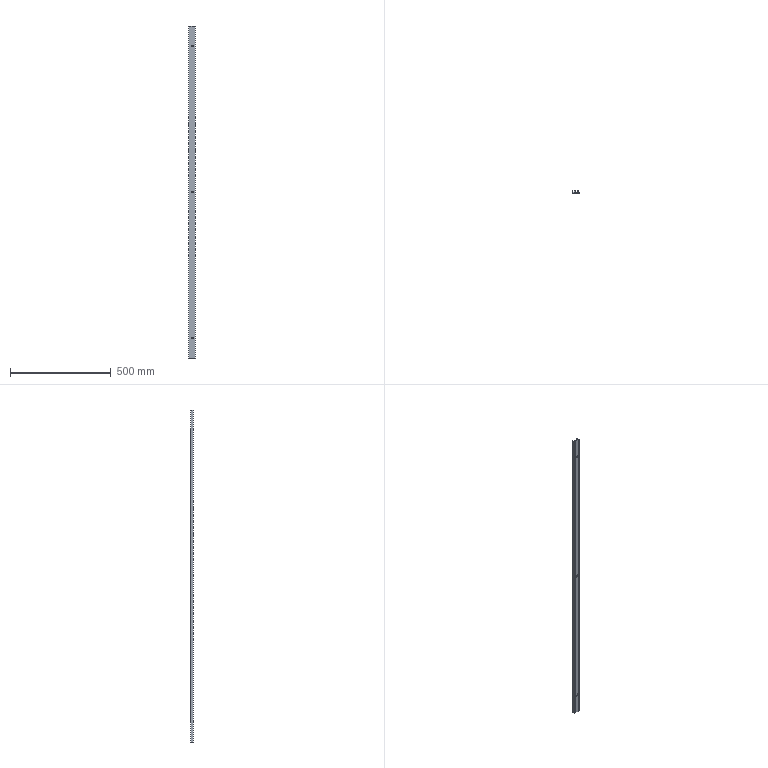Part | SolidWorks | features BaseBody 1, HoleWzd 1, ICE 1, MoveFace 1 | 1 solid | 31 faces | box 33.5 x 13.5 x 1650 mm | volume 308881 mm3 | plane 16 | cylinder 9 | cone 6 | commonest cylinder face diameters 2 x3 13.44 x3 4 x2 1.5 x1
STEP:
#1=CARTESIAN_POINT('',(20.,0.,1453.72));
#2=VERTEX_POINT('',#1);
#3=CARTESIAN_POINT('',(20.,0.,1446.28));
#4=VERTEX_POINT('',#3);
#5=CARTESIAN_POINT('',(20.,0.,1450.));
#6=DIRECTION('',(0.,-1.,0.));
#7=DIRECTION('',(0.,0.,-1.));
#8=AXIS2_PLACEMENT_3D('',#5,#6,#7);
#9=CIRCLE('',#8,3.72);
#10=EDGE_CURVE('',#2,#4,#9,.T.);
#11=ORIENTED_EDGE('',*,*,#10,.T.);
#12=CARTESIAN_POINT('',(20.,3.,1443.28));
#13=VERTEX_POINT('',#12);
#14=CARTESIAN_POINT('',(20.,3.,1443.28));
#15=DIRECTION('',(0.,0.7071,-0.7071));
#16=VECTOR('',#15,1000.);
#17=LINE('',#14,#16);
#18=EDGE_CURVE('',#4,#13,#17,.T.);
#19=ORIENTED_EDGE('',*,*,#18,.T.);
#20=CARTESIAN_POINT('',(20.,3.,1456.72));
#21=VERTEX_POINT('',#20);
#22=CARTESIAN_POINT('',(20.,3.,1450.));
#23=DIRECTION('',(0.,1.,0.));
#24=DIRECTION('',(0.,0.,1.));
#25=AXIS2_PLACEMENT_3D('',#22,#23,#24);
#26=CIRCLE('',#25,6.72);
#27=EDGE_CURVE('',#13,#21,#26,.T.);
#28=ORIENTED_EDGE('',*,*,#27,.T.);
#29=CARTESIAN_POINT('',(20.,3.,1456.72));
#30=DIRECTION('',(0.,0.7071,0.7071));
#31=VECTOR('',#30,1000.);
#32=LINE('',#29,#31);
#33=EDGE_CURVE('',#2,#21,#32,.T.);
#34=ORIENTED_EDGE('',*,*,#33,.F.);
#35=EDGE_LOOP('',(#11,#19,#28,#34));
#36=FACE_OUTER_BOUND('',#35,.T.);
#37=CARTESIAN_POINT('',(20.,3.,1450.));
#38=DIRECTION('',(0.,1.,0.));
#39=DIRECTION('',(0.,0.,1.));
#40=AXIS2_PLACEMENT_3D('',#37,#38,#39);
#41=CONICAL_SURFACE('',#40,6.72,0.7854);
#42=ADVANCED_FACE('',(#36),#41,.F.);
#43=CARTESIAN_POINT('',(20.,0.,3.72));
#44=VERTEX_POINT('',#43);
#45=CARTESIAN_POINT('',(20.,0.,-3.72));
#46=VERTEX_POINT('',#45);
#47=CARTESIAN_POINT('',(20.,0.,0.));
#48=DIRECTION('',(0.,-1.,0.));
#49=DIRECTION('',(0.,0.,-1.));
#50=AXIS2_PLACEMENT_3D('',#47,#48,#49);
#51=CIRCLE('',#50,3.72);
#52=EDGE_CURVE('',#44,#46,#51,.T.);
#53=ORIENTED_EDGE('',*,*,#52,.T.);
#54=CARTESIAN_POINT('',(20.,3.,-6.72));
#55=VERTEX_POINT('',#54);
#56=CARTESIAN_POINT('',(20.,3.,-6.72));
#57=DIRECTION('',(0.,0.7071,-0.7071));
#58=VECTOR('',#57,1000.);
#59=LINE('',#56,#58);
#60=EDGE_CURVE('',#46,#55,#59,.T.);
#61=ORIENTED_EDGE('',*,*,#60,.T.);
#62=CARTESIAN_POINT('',(20.,3.,6.72));
#63=VERTEX_POINT('',#62);
#64=CARTESIAN_POINT('',(20.,3.,0.));
#65=DIRECTION('',(0.,1.,0.));
#66=DIRECTION('',(0.,0.,1.));
#67=AXIS2_PLACEMENT_3D('',#64,#65,#66);
#68=CIRCLE('',#67,6.72);
#69=EDGE_CURVE('',#55,#63,#68,.T.);
#70=ORIENTED_EDGE('',*,*,#69,.T.);
#71=CARTESIAN_POINT('',(20.,3.,6.72));
#72=DIRECTION('',(0.,0.7071,0.7071));
#73=VECTOR('',#72,1000.);
#74=LINE('',#71,#73);
#75=EDGE_CURVE('',#44,#63,#74,.T.);
#76=ORIENTED_EDGE('',*,*,#75,.F.);
#77=EDGE_LOOP('',(#53,#61,#70,#76));
#78=FACE_OUTER_BOUND('',#77,.T.);
#79=CARTESIAN_POINT('',(20.,3.,0.));
#80=DIRECTION('',(0.,1.,0.));
#81=DIRECTION('',(0.,0.,1.));
#82=AXIS2_PLACEMENT_3D('',#79,#80,#81);
#83=CONICAL_SURFACE('',#82,6.72,0.7854);
#84=ADVANCED_FACE('',(#78),#83,.F.);
#85=CARTESIAN_POINT('',(20.,0.,728.72));
#86=VERTEX_POINT('',#85);
#87=CARTESIAN_POINT('',(20.,0.,721.28));
#88=VERTEX_POINT('',#87);
#89=CARTESIAN_POINT('',(20.,0.,725.));
#90=DIRECTION('',(0.,-1.,0.));
#91=DIRECTION('',(0.,0.,-1.));
#92=AXIS2_PLACEMENT_3D('',#89,#90,#91);
#93=CIRCLE('',#92,3.72);
#94=EDGE_CURVE('',#86,#88,#93,.T.);
#95=ORIENTED_EDGE('',*,*,#94,.T.);
#96=CARTESIAN_POINT('',(20.,3.,718.28));
#97=VERTEX_POINT('',#96);
#98=CARTESIAN_POINT('',(20.,3.,718.28));
#99=DIRECTION('',(0.,0.7071,-0.7071));
#100=VECTOR('',#99,1000.);
#101=LINE('',#98,#100);
#102=EDGE_CURVE('',#88,#97,#101,.T.);
#103=ORIENTED_EDGE('',*,*,#102,.T.);
#104=CARTESIAN_POINT('',(20.,3.,731.72));
#105=VERTEX_POINT('',#104);
#106=CARTESIAN_POINT('',(20.,3.,725.));
#107=DIRECTION('',(0.,1.,0.));
#108=DIRECTION('',(0.,0.,1.));
#109=AXIS2_PLACEMENT_3D('',#106,#107,#108);
#110=CIRCLE('',#109,6.72);
#111=EDGE_CURVE('',#97,#105,#110,.T.);
#112=ORIENTED_EDGE('',*,*,#111,.T.);
#113=CARTESIAN_POINT('',(20.,3.,731.72));
#114=DIRECTION('',(0.,0.7071,0.7071));
#115=VECTOR('',#114,1000.);
#116=LINE('',#113,#115);
#117=EDGE_CURVE('',#86,#105,#116,.T.);
#118=ORIENTED_EDGE('',*,*,#117,.F.);
#119=EDGE_LOOP('',(#95,#103,#112,#118));
#120=FACE_OUTER_BOUND('',#119,.T.);
#121=CARTESIAN_POINT('',(20.,3.,725.));
#122=DIRECTION('',(0.,1.,0.));
#123=DIRECTION('',(0.,0.,1.));
#124=AXIS2_PLACEMENT_3D('',#121,#122,#123);
#125=CONICAL_SURFACE('',#124,6.72,0.7854);
#126=ADVANCED_FACE('',(#120),#125,.F.);
#127=CARTESIAN_POINT('',(24.5,10.5,-4.991));
#128=VERTEX_POINT('',#127);
#129=CARTESIAN_POINT('',(24.5,10.5,-100.));
#130=VERTEX_POINT('',#129);
#131=CARTESIAN_POINT('',(24.5,10.5,-100.));
#132=DIRECTION('',(0.,0.,-1.));
#133=VECTOR('',#132,1000.);
#134=LINE('',#131,#133);
#135=EDGE_CURVE('',#128,#130,#134,.T.);
#136=ORIENTED_EDGE('',*,*,#135,.F.);
#137=CARTESIAN_POINT('',(24.5,10.5,4.991));
#138=VERTEX_POINT('',#137);
#139=CARTESIAN_POINT('',(24.5,10.5,-4.991));
#140=CARTESIAN_POINT('',(24.5,10.638,-4.991));
#141=CARTESIAN_POINT('',(24.515,10.777,-4.978));
#142=CARTESIAN_POINT('',(24.57,11.043,-4.927));
#143=CARTESIAN_POINT('',(24.611,11.171,-4.889));
#144=CARTESIAN_POINT('',(24.765,11.529,-4.74));
#145=CARTESIAN_POINT('',(24.907,11.728,-4.597));
#146=CARTESIAN_POINT('',(25.205,12.04,-4.256));
#147=CARTESIAN_POINT('',(25.365,12.156,-4.055));
#148=CARTESIAN_POINT('',(25.663,12.325,-3.627));
#149=CARTESIAN_POINT('',(25.806,12.38,-3.395));
#150=CARTESIAN_POINT('',(26.19,12.494,-2.672));
#151=CARTESIAN_POINT('',(26.387,12.501,-2.161));
#152=CARTESIAN_POINT('',(26.654,12.499,-1.091));
#153=CARTESIAN_POINT('',(26.72,12.488,-0.5481));
#154=CARTESIAN_POINT('',(26.72,12.488,0.2773));
#155=CARTESIAN_POINT('',(26.703,12.49,0.5529));
#156=CARTESIAN_POINT('',(26.636,12.496,1.095));
#157=CARTESIAN_POINT('',(26.586,12.499,1.362));
#158=CARTESIAN_POINT('',(26.388,12.501,2.155));
#159=CARTESIAN_POINT('',(26.188,12.493,2.677));
#160=CARTESIAN_POINT('',(25.805,12.38,3.396));
#161=CARTESIAN_POINT('',(25.662,12.324,3.629));
#162=CARTESIAN_POINT('',(25.438,12.197,3.95));
#163=CARTESIAN_POINT('',(25.362,12.147,4.053));
#164=CARTESIAN_POINT('',(25.208,12.03,4.249));
#165=CARTESIAN_POINT('',(25.13,11.961,4.342));
#166=CARTESIAN_POINT('',(24.98,11.805,4.513));
#167=CARTESIAN_POINT('',(24.908,11.717,4.591));
#168=CARTESIAN_POINT('',(24.774,11.518,4.73));
#169=CARTESIAN_POINT('',(24.714,11.408,4.79));
#170=CARTESIAN_POINT('',(24.612,11.172,4.888));
#171=CARTESIAN_POINT('',(24.57,11.043,4.927));
#172=CARTESIAN_POINT('',(24.515,10.778,4.978));
#173=CARTESIAN_POINT('',(24.5,10.64,4.991));
#174=CARTESIAN_POINT('',(24.5,10.5,4.991));
#175=B_SPLINE_CURVE_WITH_KNOTS('',3,(#139,#140,#141,#142,#143,#144,#145,#146,#147,#148,#149,#150,#151,#152,#153,#154,#155,#156,#157,#158,#159,#160,#161,#162,#163,#164,#165,#166,#167,#168,#169,#170,#171,#172,#173,#174),.UNSPECIFIED.,.F.,.F.,(4,2,2,2,2,2,2,2,2,2,2,2,2,2,2,2,2,4),(0.01321,0.01362,0.01403,0.01486,0.01569,0.01651,0.01816,0.01981,0.02064,0.02146,0.02311,0.02394,0.02435,0.02477,0.02518,0.02559,0.026,0.02642),.UNSPECIFIED.);
#176=EDGE_CURVE('',#128,#138,#175,.T.);
#177=ORIENTED_EDGE('',*,*,#176,.T.);
#178=CARTESIAN_POINT('',(24.5,10.5,720.009));
#179=VERTEX_POINT('',#178);
#180=CARTESIAN_POINT('',(24.5,10.5,-100.));
#181=DIRECTION('',(0.,0.,-1.));
#182=VECTOR('',#181,1000.);
#183=LINE('',#180,#182);
#184=EDGE_CURVE('',#179,#138,#183,.T.);
#185=ORIENTED_EDGE('',*,*,#184,.F.);
#186=CARTESIAN_POINT('',(24.5,10.5,729.991));
#187=VERTEX_POINT('',#186);
#188=CARTESIAN_POINT('',(24.5,10.5,720.009));
#189=CARTESIAN_POINT('',(24.5,10.638,720.009));
#190=CARTESIAN_POINT('',(24.515,10.777,720.022));
#191=CARTESIAN_POINT('',(24.57,11.043,720.073));
#192=CARTESIAN_POINT('',(24.611,11.171,720.111));
#193=CARTESIAN_POINT('',(24.765,11.529,720.26));
#194=CARTESIAN_POINT('',(24.907,11.728,720.403));
#195=CARTESIAN_POINT('',(25.205,12.04,720.744));
#196=CARTESIAN_POINT('',(25.365,12.156,720.945));
#197=CARTESIAN_POINT('',(25.663,12.325,721.373));
#198=CARTESIAN_POINT('',(25.806,12.38,721.605));
#199=CARTESIAN_POINT('',(26.19,12.494,722.328));
#200=CARTESIAN_POINT('',(26.387,12.501,722.839));
#201=CARTESIAN_POINT('',(26.654,12.499,723.909));
#202=CARTESIAN_POINT('',(26.72,12.488,724.452));
#203=CARTESIAN_POINT('',(26.72,12.488,725.277));
#204=CARTESIAN_POINT('',(26.703,12.49,725.553));
#205=CARTESIAN_POINT('',(26.636,12.496,726.095));
#206=CARTESIAN_POINT('',(26.586,12.499,726.362));
#207=CARTESIAN_POINT('',(26.388,12.501,727.155));
#208=CARTESIAN_POINT('',(26.188,12.493,727.677));
#209=CARTESIAN_POINT('',(25.805,12.38,728.396));
#210=CARTESIAN_POINT('',(25.662,12.324,728.629));
#211=CARTESIAN_POINT('',(25.438,12.197,728.95));
#212=CARTESIAN_POINT('',(25.362,12.147,729.053));
#213=CARTESIAN_POINT('',(25.208,12.03,729.249));
#214=CARTESIAN_POINT('',(25.13,11.961,729.342));
#215=CARTESIAN_POINT('',(24.98,11.805,729.513));
#216=CARTESIAN_POINT('',(24.908,11.717,729.591));
#217=CARTESIAN_POINT('',(24.774,11.518,729.73));
#218=CARTESIAN_POINT('',(24.714,11.408,729.79));
#219=CARTESIAN_POINT('',(24.612,11.172,729.888));
#220=CARTESIAN_POINT('',(24.57,11.043,729.927));
#221=CARTESIAN_POINT('',(24.515,10.778,729.978));
#222=CARTESIAN_POINT('',(24.5,10.64,729.991));
#223=CARTESIAN_POINT('',(24.5,10.5,729.991));
#224=B_SPLINE_CURVE_WITH_KNOTS('',3,(#188,#189,#190,#191,#192,#193,#194,#195,#196,#197,#198,#199,#200,#201,#202,#203,#204,#205,#206,#207,#208,#209,#210,#211,#212,#213,#214,#215,#216,#217,#218,#219,#220,#221,#222,#223),.UNSPECIFIED.,.F.,.F.,(4,2,2,2,2,2,2,2,2,2,2,2,2,2,2,2,2,4),(0.01321,0.01362,0.01403,0.01486,0.01569,0.01651,0.01816,0.01981,0.02064,0.02146,0.02311,0.02394,0.02435,0.02477,0.02518,0.02559,0.026,0.02642),.UNSPECIFIED.);
#225=EDGE_CURVE('',#179,#187,#224,.T.);
#226=ORIENTED_EDGE('',*,*,#225,.T.);
#227=CARTESIAN_POINT('',(24.5,10.5,1445.009));
#228=VERTEX_POINT('',#227);
#229=CARTESIAN_POINT('',(24.5,10.5,-100.));
#230=DIRECTION('',(0.,0.,-1.));
#231=VECTOR('',#230,1000.);
#232=LINE('',#229,#231);
#233=EDGE_CURVE('',#228,#187,#232,.T.);
#234=ORIENTED_EDGE('',*,*,#233,.F.);
#235=CARTESIAN_POINT('',(24.5,10.5,1454.991));
#236=VERTEX_POINT('',#235);
#237=CARTESIAN_POINT('',(24.5,10.5,1445.009));
#238=CARTESIAN_POINT('',(24.5,10.64,1445.009));
#239=CARTESIAN_POINT('',(24.514,10.776,1445.022));
#240=CARTESIAN_POINT('',(24.57,11.042,1445.073));
#241=CARTESIAN_POINT('',(24.611,11.171,1445.111));
#242=CARTESIAN_POINT('',(24.713,11.408,1445.209));
#243=CARTESIAN_POINT('',(24.775,11.519,1445.27));
#244=CARTESIAN_POINT('',(24.908,11.717,1445.409));
#245=CARTESIAN_POINT('',(24.981,11.806,1445.488));
#246=CARTESIAN_POINT('',(25.207,12.042,1445.746));
#247=CARTESIAN_POINT('',(25.363,12.155,1445.942));
#248=CARTESIAN_POINT('',(25.665,12.326,1446.376));
#249=CARTESIAN_POINT('',(25.806,12.38,1446.605));
#250=CARTESIAN_POINT('',(26.061,12.456,1447.084));
#251=CARTESIAN_POINT('',(26.176,12.476,1447.337));
#252=CARTESIAN_POINT('',(26.372,12.498,1447.849));
#253=CARTESIAN_POINT('',(26.454,12.501,1448.109));
#254=CARTESIAN_POINT('',(26.586,12.499,1448.638));
#255=CARTESIAN_POINT('',(26.636,12.496,1448.907));
#256=CARTESIAN_POINT('',(26.703,12.49,1449.453));
#257=CARTESIAN_POINT('',(26.72,12.488,1449.729));
#258=CARTESIAN_POINT('',(26.72,12.488,1450.275));
#259=CARTESIAN_POINT('',(26.703,12.49,1450.547));
#260=CARTESIAN_POINT('',(26.637,12.496,1451.089));
#261=CARTESIAN_POINT('',(26.587,12.499,1451.36));
#262=CARTESIAN_POINT('',(26.387,12.501,1452.161));
#263=CARTESIAN_POINT('',(26.191,12.494,1452.671));
#264=CARTESIAN_POINT('',(25.805,12.38,1453.396));
#265=CARTESIAN_POINT('',(25.663,12.325,1453.627));
#266=CARTESIAN_POINT('',(25.364,12.155,1454.057));
#267=CARTESIAN_POINT('',(25.205,12.039,1454.256));
#268=CARTESIAN_POINT('',(24.981,11.805,1454.512));
#269=CARTESIAN_POINT('',(24.907,11.716,1454.592));
#270=CARTESIAN_POINT('',(24.774,11.518,1454.73));
#271=CARTESIAN_POINT('',(24.714,11.409,1454.79));
#272=CARTESIAN_POINT('',(24.611,11.17,1454.889));
#273=CARTESIAN_POINT('',(24.571,11.044,1454.926));
#274=CARTESIAN_POINT('',(24.515,10.78,1454.977));
#275=CARTESIAN_POINT('',(24.5,10.64,1454.991));
#276=CARTESIAN_POINT('',(24.5,10.5,1454.991));
#277=B_SPLINE_CURVE_WITH_KNOTS('',3,(#237,#238,#239,#240,#241,#242,#243,#244,#245,#246,#247,#248,#249,#250,#251,#252,#253,#254,#255,#256,#257,#258,#259,#260,#261,#262,#263,#264,#265,#266,#267,#268,#269,#270,#271,#272,#273,#274,#275,#276),.UNSPECIFIED.,.F.,.F.,(4,2,2,2,2,2,2,2,2,2,2,2,2,2,2,2,2,2,2,4),(0.,0.0004127,0.0008255,0.001238,0.001651,0.002476,0.003302,0.004127,0.004953,0.005778,0.006604,0.007429,0.008255,0.009906,0.01073,0.01156,0.01197,0.01238,0.01279,0.01321),.UNSPECIFIED.);
#278=EDGE_CURVE('',#228,#236,#277,.T.);
#279=ORIENTED_EDGE('',*,*,#278,.T.);
#280=CARTESIAN_POINT('',(24.5,10.5,1550.));
#281=VERTEX_POINT('',#280);
#282=CARTESIAN_POINT('',(24.5,10.5,-100.));
#283=DIRECTION('',(0.,0.,-1.));
#284=VECTOR('',#283,1000.);
#285=LINE('',#282,#284);
#286=EDGE_CURVE('',#281,#236,#285,.T.);
#287=ORIENTED_EDGE('',*,*,#286,.F.);
#288=CARTESIAN_POINT('',(28.5,10.5,1550.));
#289=VERTEX_POINT('',#288);
#290=CARTESIAN_POINT('',(26.5,10.5,1550.));
#291=DIRECTION('',(0.,0.,1.));
#292=DIRECTION('',(1.,0.,0.));
#293=AXIS2_PLACEMENT_3D('',#290,#291,#292);
#294=CIRCLE('',#293,2.);
#295=EDGE_CURVE('',#289,#281,#294,.T.);
#296=ORIENTED_EDGE('',*,*,#295,.F.);
#297=CARTESIAN_POINT('',(28.5,10.5,-100.));
#298=VERTEX_POINT('',#297);
#299=CARTESIAN_POINT('',(28.5,10.5,-100.));
#300=DIRECTION('',(0.,0.,-1.));
#301=VECTOR('',#300,1000.);
#302=LINE('',#299,#301);
#303=EDGE_CURVE('',#289,#298,#302,.T.);
#304=ORIENTED_EDGE('',*,*,#303,.T.);
#305=CARTESIAN_POINT('',(26.5,10.5,-100.));
#306=DIRECTION('',(0.,0.,1.));
#307=DIRECTION('',(-1.,0.,0.));
#308=AXIS2_PLACEMENT_3D('',#305,#306,#307);
#309=CIRCLE('',#308,2.);
#310=EDGE_CURVE('',#298,#130,#309,.T.);
#311=ORIENTED_EDGE('',*,*,#310,.T.);
#312=EDGE_LOOP('',(#136,#177,#185,#226,#234,#279,#287,#296,#304,#311));
#313=FACE_OUTER_BOUND('',#312,.T.);
#314=CARTESIAN_POINT('',(26.5,10.5,-100.));
#315=DIRECTION('',(0.,0.,-1.));
#316=DIRECTION('',(-1.,0.,0.));
#317=AXIS2_PLACEMENT_3D('',#314,#315,#316);
#318=CYLINDRICAL_SURFACE('',#317,2.);
#319=ADVANCED_FACE('',(#313),#318,.T.);
#320=CARTESIAN_POINT('',(24.5,3.,-4.991));
#321=VERTEX_POINT('',#320);
#322=CARTESIAN_POINT('',(24.5,3.,-100.));
#323=VERTEX_POINT('',#322);
#324=CARTESIAN_POINT('',(24.5,3.,-100.));
#325=DIRECTION('',(0.,0.,-1.));
#326=VECTOR('',#325,1000.);
#327=LINE('',#324,#326);
#328=EDGE_CURVE('',#321,#323,#327,.T.);
#329=ORIENTED_EDGE('',*,*,#328,.F.);
#330=CARTESIAN_POINT('',(24.5,13.5,-4.991));
#331=DIRECTION('',(0.,1.,0.));
#332=VECTOR('',#331,1000.);
#333=LINE('',#330,#332);
#334=EDGE_CURVE('',#321,#128,#333,.T.);
#335=ORIENTED_EDGE('',*,*,#334,.T.);
#336=ORIENTED_EDGE('',*,*,#135,.T.);
#337=CARTESIAN_POINT('',(24.5,1.,-100.));
#338=DIRECTION('',(0.,-1.,0.));
#339=VECTOR('',#338,1000.);
#340=LINE('',#337,#339);
#341=EDGE_CURVE('',#130,#323,#340,.T.);
#342=ORIENTED_EDGE('',*,*,#341,.T.);
#343=EDGE_LOOP('',(#329,#335,#336,#342));
#344=FACE_OUTER_BOUND('',#343,.T.);
#345=CARTESIAN_POINT('',(24.5,10.5,-100.));
#346=DIRECTION('',(-1.,0.,0.));
#347=DIRECTION('',(0.,0.,1.));
#348=AXIS2_PLACEMENT_3D('',#345,#346,#347);
#349=PLANE('',#348);
#350=ADVANCED_FACE('',(#344),#349,.T.);
#351=ORIENTED_EDGE('',*,*,#184,.T.);
#352=CARTESIAN_POINT('',(24.5,3.,4.991));
#353=VERTEX_POINT('',#352);
#354=CARTESIAN_POINT('',(24.5,13.5,4.991));
#355=DIRECTION('',(0.,-1.,0.));
#356=VECTOR('',#355,1000.);
#357=LINE('',#354,#356);
#358=EDGE_CURVE('',#138,#353,#357,.T.);
#359=ORIENTED_EDGE('',*,*,#358,.T.);
#360=CARTESIAN_POINT('',(24.5,3.,720.009));
#361=VERTEX_POINT('',#360);
#362=CARTESIAN_POINT('',(24.5,3.,-100.));
#363=DIRECTION('',(0.,0.,-1.));
#364=VECTOR('',#363,1000.);
#365=LINE('',#362,#364);
#366=EDGE_CURVE('',#361,#353,#365,.T.);
#367=ORIENTED_EDGE('',*,*,#366,.F.);
#368=CARTESIAN_POINT('',(24.5,13.5,720.009));
#369=DIRECTION('',(0.,1.,0.));
#370=VECTOR('',#369,1000.);
#371=LINE('',#368,#370);
#372=EDGE_CURVE('',#361,#179,#371,.T.);
#373=ORIENTED_EDGE('',*,*,#372,.T.);
#374=EDGE_LOOP('',(#351,#359,#367,#373));
#375=FACE_OUTER_BOUND('',#374,.T.);
#376=CARTESIAN_POINT('',(24.5,10.5,-100.));
#377=DIRECTION('',(-1.,0.,0.));
#378=DIRECTION('',(0.,0.,1.));
#379=AXIS2_PLACEMENT_3D('',#376,#377,#378);
#380=PLANE('',#379);
#381=ADVANCED_FACE('',(#375),#380,.T.);
#382=ORIENTED_EDGE('',*,*,#233,.T.);
#383=CARTESIAN_POINT('',(24.5,3.,729.991));
#384=VERTEX_POINT('',#383);
#385=CARTESIAN_POINT('',(24.5,13.5,729.991));
#386=DIRECTION('',(0.,-1.,0.));
#387=VECTOR('',#386,1000.);
#388=LINE('',#385,#387);
#389=EDGE_CURVE('',#187,#384,#388,.T.);
#390=ORIENTED_EDGE('',*,*,#389,.T.);
#391=CARTESIAN_POINT('',(24.5,3.,1445.009));
#392=VERTEX_POINT('',#391);
#393=CARTESIAN_POINT('',(24.5,3.,-100.));
#394=DIRECTION('',(0.,0.,-1.));
#395=VECTOR('',#394,1000.);
#396=LINE('',#393,#395);
#397=EDGE_CURVE('',#392,#384,#396,.T.);
#398=ORIENTED_EDGE('',*,*,#397,.F.);
#399=CARTESIAN_POINT('',(24.5,13.5,1445.009));
#400=DIRECTION('',(0.,1.,0.));
#401=VECTOR('',#400,1000.);
#402=LINE('',#399,#401);
#403=EDGE_CURVE('',#392,#228,#402,.T.);
#404=ORIENTED_EDGE('',*,*,#403,.T.);
#405=EDGE_LOOP('',(#382,#390,#398,#404));
#406=FACE_OUTER_BOUND('',#405,.T.);
#407=CARTESIAN_POINT('',(24.5,10.5,-100.));
#408=DIRECTION('',(-1.,0.,0.));
#409=DIRECTION('',(0.,0.,1.));
#410=AXIS2_PLACEMENT_3D('',#407,#408,#409);
#411=PLANE('',#410);
#412=ADVANCED_FACE('',(#406),#411,.T.);
#413=ORIENTED_EDGE('',*,*,#286,.T.);
#414=CARTESIAN_POINT('',(24.5,3.,1454.991));
#415=VERTEX_POINT('',#414);
#416=CARTESIAN_POINT('',(24.5,13.5,1454.991));
#417=DIRECTION('',(0.,-1.,0.));
#418=VECTOR('',#417,1000.);
#419=LINE('',#416,#418);
#420=EDGE_CURVE('',#236,#415,#419,.T.);
#421=ORIENTED_EDGE('',*,*,#420,.T.);
#422=CARTESIAN_POINT('',(24.5,3.,1550.));
#423=VERTEX_POINT('',#422);
#424=CARTESIAN_POINT('',(24.5,3.,-100.));
#425=DIRECTION('',(0.,0.,-1.));
#426=VECTOR('',#425,1000.);
#427=LINE('',#424,#426);
#428=EDGE_CURVE('',#423,#415,#427,.T.);
#429=ORIENTED_EDGE('',*,*,#428,.F.);
#430=CARTESIAN_POINT('',(24.5,1.,1550.));
#431=DIRECTION('',(0.,-1.,0.));
#432=VECTOR('',#431,1000.);
#433=LINE('',#430,#432);
#434=EDGE_CURVE('',#281,#423,#433,.T.);
#435=ORIENTED_EDGE('',*,*,#434,.F.);
#436=EDGE_LOOP('',(#413,#421,#429,#435));
#437=FACE_OUTER_BOUND('',#436,.T.);
#438=CARTESIAN_POINT('',(24.5,10.5,-100.));
#439=DIRECTION('',(-1.,0.,0.));
#440=DIRECTION('',(0.,0.,1.));
#441=AXIS2_PLACEMENT_3D('',#438,#439,#440);
#442=PLANE('',#441);
#443=ADVANCED_FACE('',(#437),#442,.T.);
#444=ORIENTED_EDGE('',*,*,#10,.F.);
#445=CARTESIAN_POINT('',(20.,0.,1450.));
#446=DIRECTION('',(0.,-1.,0.));
#447=DIRECTION('',(0.,0.,-1.));
#448=AXIS2_PLACEMENT_3D('',#445,#446,#447);
#449=CIRCLE('',#448,3.72);
#450=EDGE_CURVE('',#4,#2,#449,.T.);
#451=ORIENTED_EDGE('',*,*,#450,.F.);
#452=EDGE_LOOP('',(#444,#451));
#453=FACE_BOUND('',#452,.T.);
#454=ORIENTED_EDGE('',*,*,#52,.F.);
#455=CARTESIAN_POINT('',(20.,0.,0.));
#456=DIRECTION('',(0.,-1.,0.));
#457=DIRECTION('',(0.,0.,-1.));
#458=AXIS2_PLACEMENT_3D('',#455,#456,#457);
#459=CIRCLE('',#458,3.72);
#460=EDGE_CURVE('',#46,#44,#459,.T.);
#461=ORIENTED_EDGE('',*,*,#460,.F.);
#462=EDGE_LOOP('',(#454,#461));
#463=FACE_BOUND('',#462,.T.);
#464=CARTESIAN_POINT('',(1.,0.,-100.));
#465=VERTEX_POINT('',#464);
#466=CARTESIAN_POINT('',(32.5,0.,-100.));
#467=VERTEX_POINT('',#466);
#468=CARTESIAN_POINT('',(1.,0.,-100.));
#469=DIRECTION('',(1.,0.,0.));
#470=VECTOR('',#469,1000.);
#471=LINE('',#468,#470);
#472=EDGE_CURVE('',#465,#467,#471,.T.);
#473=ORIENTED_EDGE('',*,*,#472,.T.);
#474=CARTESIAN_POINT('',(32.5,0.,1550.));
#475=VERTEX_POINT('',#474);
#476=CARTESIAN_POINT('',(32.5,0.,-100.));
#477=DIRECTION('',(0.,0.,1.));
#478=VECTOR('',#477,1000.);
#479=LINE('',#476,#478);
#480=EDGE_CURVE('',#467,#475,#479,.T.);
#481=ORIENTED_EDGE('',*,*,#480,.T.);
#482=CARTESIAN_POINT('',(1.,0.,1550.));
#483=VERTEX_POINT('',#482);
#484=CARTESIAN_POINT('',(1.,0.,1550.));
#485=DIRECTION('',(-1.,0.,0.));
#486=VECTOR('',#485,1000.);
#487=LINE('',#484,#486);
#488=EDGE_CURVE('',#475,#483,#487,.T.);
#489=ORIENTED_EDGE('',*,*,#488,.T.);
#490=CARTESIAN_POINT('',(1.,0.,-100.));
#491=DIRECTION('',(0.,0.,-1.));
#492=VECTOR('',#491,1000.);
#493=LINE('',#490,#492);
#494=EDGE_CURVE('',#483,#465,#493,.T.);
#495=ORIENTED_EDGE('',*,*,#494,.T.);
#496=EDGE_LOOP('',(#473,#481,#489,#495));
#497=FACE_OUTER_BOUND('',#496,.T.);
#498=ORIENTED_EDGE('',*,*,#94,.F.);
#499=CARTESIAN_POINT('',(20.,0.,725.));
#500=DIRECTION('',(0.,-1.,0.));
#501=DIRECTION('',(0.,0.,-1.));
#502=AXIS2_PLACEMENT_3D('',#499,#500,#501);
#503=CIRCLE('',#502,3.72);
#504=EDGE_CURVE('',#88,#86,#503,.T.);
#505=ORIENTED_EDGE('',*,*,#504,.F.);
#506=EDGE_LOOP('',(#498,#505));
#507=FACE_BOUND('',#506,.T.);
#508=CARTESIAN_POINT('',(1.,0.,-100.));
#509=DIRECTION('',(0.,-1.,0.));
#510=DIRECTION('',(0.,0.,-1.));
#511=AXIS2_PLACEMENT_3D('',#508,#509,#510);
#512=PLANE('',#511);
#513=ADVANCED_FACE('',(#453,#463,#497,#507),#512,.T.);
#514=CARTESIAN_POINT('',(33.5,1.,-100.));
#515=VERTEX_POINT('',#514);
#516=CARTESIAN_POINT('',(32.5,1.,-100.));
#517=DIRECTION('',(0.,0.,1.));
#518=DIRECTION('',(-1.,0.,0.));
#519=AXIS2_PLACEMENT_3D('',#516,#517,#518);
#520=CIRCLE('',#519,1.);
#521=EDGE_CURVE('',#467,#515,#520,.T.);
#522=ORIENTED_EDGE('',*,*,#521,.T.);
#523=CARTESIAN_POINT('',(33.5,1.,1550.));
#524=VERTEX_POINT('',#523);
#525=CARTESIAN_POINT('',(33.5,1.,-100.));
#526=DIRECTION('',(0.,0.,1.));
#527=VECTOR('',#526,1000.);
#528=LINE('',#525,#527);
#529=EDGE_CURVE('',#515,#524,#528,.T.);
#530=ORIENTED_EDGE('',*,*,#529,.T.);
#531=CARTESIAN_POINT('',(32.5,1.,1550.));
#532=DIRECTION('',(0.,0.,-1.));
#533=DIRECTION('',(1.,0.,0.));
#534=AXIS2_PLACEMENT_3D('',#531,#532,#533);
#535=CIRCLE('',#534,1.);
#536=EDGE_CURVE('',#524,#475,#535,.T.);
#537=ORIENTED_EDGE('',*,*,#536,.T.);
#538=ORIENTED_EDGE('',*,*,#480,.F.);
#539=EDGE_LOOP('',(#522,#530,#537,#538));
#540=FACE_OUTER_BOUND('',#539,.T.);
#541=CARTESIAN_POINT('',(32.5,1.,-100.));
#542=DIRECTION('',(0.,0.,-1.));
#543=DIRECTION('',(-1.,0.,0.));
#544=AXIS2_PLACEMENT_3D('',#541,#542,#543);
#545=CYLINDRICAL_SURFACE('',#544,1.);
#546=ADVANCED_FACE('',(#540),#545,.T.);
#547=CARTESIAN_POINT('',(1.5,12.75,-100.));
#548=VERTEX_POINT('',#547);
#549=CARTESIAN_POINT('',(0.,12.75,-100.));
#550=VERTEX_POINT('',#549);
#551=CARTESIAN_POINT('',(0.75,12.75,-100.));
#552=DIRECTION('',(0.,0.,1.));
#553=DIRECTION('',(-1.,0.,0.));
#554=AXIS2_PLACEMENT_3D('',#551,#552,#553);
#555=CIRCLE('',#554,0.75);
#556=EDGE_CURVE('',#548,#550,#555,.T.);
#557=ORIENTED_EDGE('',*,*,#556,.F.);
#558=CARTESIAN_POINT('',(1.5,3.,-100.));
#559=VERTEX_POINT('',#558);
#560=CARTESIAN_POINT('',(1.5,1.,-100.));
#561=DIRECTION('',(0.,1.,0.));
#562=VECTOR('',#561,1000.);
#563=LINE('',#560,#562);
#564=EDGE_CURVE('',#559,#548,#563,.T.);
#565=ORIENTED_EDGE('',*,*,#564,.F.);
#566=CARTESIAN_POINT('',(8.5,3.,-100.));
#567=VERTEX_POINT('',#566);
#568=CARTESIAN_POINT('',(1.,3.,-100.));
#569=DIRECTION('',(-1.,0.,0.));
#570=VECTOR('',#569,1000.);
#571=LINE('',#568,#570);
#572=EDGE_CURVE('',#567,#559,#571,.T.);
#573=ORIENTED_EDGE('',*,*,#572,.F.);
#574=CARTESIAN_POINT('',(8.5,10.5,-100.));
#575=VERTEX_POINT('',#574);
#576=CARTESIAN_POINT('',(8.5,1.,-100.));
#577=DIRECTION('',(0.,-1.,0.));
#578=VECTOR('',#577,1000.);
#579=LINE('',#576,#578);
#580=EDGE_CURVE('',#575,#567,#579,.T.);
#581=ORIENTED_EDGE('',*,*,#580,.F.);
#582=CARTESIAN_POINT('',(12.5,10.5,-100.));
#583=VERTEX_POINT('',#582);
#584=CARTESIAN_POINT('',(10.5,10.5,-100.));
#585=DIRECTION('',(0.,0.,1.));
#586=DIRECTION('',(-1.,0.,0.));
#587=AXIS2_PLACEMENT_3D('',#584,#585,#586);
#588=CIRCLE('',#587,2.);
#589=EDGE_CURVE('',#583,#575,#588,.T.);
#590=ORIENTED_EDGE('',*,*,#589,.F.);
#591=CARTESIAN_POINT('',(12.5,3.,-100.));
#592=VERTEX_POINT('',#591);
#593=CARTESIAN_POINT('',(12.5,1.,-100.));
#594=DIRECTION('',(0.,1.,0.));
#595=VECTOR('',#594,1000.);
#596=LINE('',#593,#595);
#597=EDGE_CURVE('',#592,#583,#596,.T.);
#598=ORIENTED_EDGE('',*,*,#597,.F.);
#599=CARTESIAN_POINT('',(1.,3.,-100.));
#600=DIRECTION('',(-1.,0.,0.));
#601=VECTOR('',#600,1000.);
#602=LINE('',#599,#601);
#603=EDGE_CURVE('',#323,#592,#602,.T.);
#604=ORIENTED_EDGE('',*,*,#603,.F.);
#605=ORIENTED_EDGE('',*,*,#341,.F.);
#606=ORIENTED_EDGE('',*,*,#310,.F.);
#607=CARTESIAN_POINT('',(28.5,3.,-100.));
#608=VERTEX_POINT('',#607);
#609=CARTESIAN_POINT('',(28.5,1.,-100.));
#610=DIRECTION('',(0.,1.,0.));
#611=VECTOR('',#610,1000.);
#612=LINE('',#609,#611);
#613=EDGE_CURVE('',#608,#298,#612,.T.);
#614=ORIENTED_EDGE('',*,*,#613,.F.);
#615=CARTESIAN_POINT('',(32.5,3.,-100.));
#616=VERTEX_POINT('',#615);
#617=CARTESIAN_POINT('',(1.,3.,-100.));
#618=DIRECTION('',(-1.,0.,0.));
#619=VECTOR('',#618,1000.);
#620=LINE('',#617,#619);
#621=EDGE_CURVE('',#616,#608,#620,.T.);
#622=ORIENTED_EDGE('',*,*,#621,.F.);
#623=CARTESIAN_POINT('',(33.5,2.,-100.));
#624=VERTEX_POINT('',#623);
#625=CARTESIAN_POINT('',(32.5,2.,-100.));
#626=DIRECTION('',(0.,0.,1.));
#627=DIRECTION('',(-1.,0.,0.));
#628=AXIS2_PLACEMENT_3D('',#625,#626,#627);
#629=CIRCLE('',#628,1.);
#630=EDGE_CURVE('',#624,#616,#629,.T.);
#631=ORIENTED_EDGE('',*,*,#630,.F.);
#632=CARTESIAN_POINT('',(33.5,1.,-100.));
#633=DIRECTION('',(0.,1.,0.));
#634=VECTOR('',#633,1000.);
#635=LINE('',#632,#634);
#636=EDGE_CURVE('',#515,#624,#635,.T.);
#637=ORIENTED_EDGE('',*,*,#636,.F.);
#638=ORIENTED_EDGE('',*,*,#521,.F.);
#639=ORIENTED_EDGE('',*,*,#472,.F.);
#640=CARTESIAN_POINT('',(0.,1.,-100.));
#641=VERTEX_POINT('',#640);
#642=CARTESIAN_POINT('',(1.,1.,-100.));
#643=DIRECTION('',(0.,0.,1.));
#644=DIRECTION('',(-1.,0.,0.));
#645=AXIS2_PLACEMENT_3D('',#642,#643,#644);
#646=CIRCLE('',#645,1.);
#647=EDGE_CURVE('',#641,#465,#646,.T.);
#648=ORIENTED_EDGE('',*,*,#647,.F.);
#649=CARTESIAN_POINT('',(0.,1.,-100.));
#650=DIRECTION('',(0.,-1.,0.));
#651=VECTOR('',#650,1000.);
#652=LINE('',#649,#651);
#653=EDGE_CURVE('',#550,#641,#652,.T.);
#654=ORIENTED_EDGE('',*,*,#653,.F.);
#655=EDGE_LOOP('',(#557,#565,#573,#581,#590,#598,#604,#605,#606,#614,#622,#631,#637,#638,#639,#648,#654));
#656=FACE_OUTER_BOUND('',#655,.T.);
#657=CARTESIAN_POINT('',(1.,1.,-100.));
#658=DIRECTION('',(0.,0.,1.));
#659=DIRECTION('',(1.,0.,0.));
#660=AXIS2_PLACEMENT_3D('',#657,#658,#659);
#661=PLANE('',#660);
#662=ADVANCED_FACE('',(#656),#661,.F.);
#663=ORIENTED_EDGE('',*,*,#647,.T.);
#664=ORIENTED_EDGE('',*,*,#494,.F.);
#665=CARTESIAN_POINT('',(0.,1.,1550.));
#666=VERTEX_POINT('',#665);
#667=CARTESIAN_POINT('',(1.,1.,1550.));
#668=DIRECTION('',(0.,0.,-1.));
#669=DIRECTION('',(1.,0.,0.));
#670=AXIS2_PLACEMENT_3D('',#667,#668,#669);
#671=CIRCLE('',#670,1.);
#672=EDGE_CURVE('',#483,#666,#671,.T.);
#673=ORIENTED_EDGE('',*,*,#672,.T.);
#674=CARTESIAN_POINT('',(0.,1.,-100.));
#675=DIRECTION('',(0.,0.,-1.));
#676=VECTOR('',#675,1000.);
#677=LINE('',#674,#676);
#678=EDGE_CURVE('',#666,#641,#677,.T.);
#679=ORIENTED_EDGE('',*,*,#678,.T.);
#680=EDGE_LOOP('',(#663,#664,#673,#679));
#681=FACE_OUTER_BOUND('',#680,.T.);
#682=CARTESIAN_POINT('',(1.,1.,-100.));
#683=DIRECTION('',(0.,0.,-1.));
#684=DIRECTION('',(-1.,0.,0.));
#685=AXIS2_PLACEMENT_3D('',#682,#683,#684);
#686=CYLINDRICAL_SURFACE('',#685,1.);
#687=ADVANCED_FACE('',(#681),#686,.T.);
#688=CARTESIAN_POINT('',(1.5,3.,1550.));
#689=VERTEX_POINT('',#688);
#690=CARTESIAN_POINT('',(1.5,12.75,1550.));
#691=VERTEX_POINT('',#690);
#692=CARTESIAN_POINT('',(1.5,1.,1550.));
#693=DIRECTION('',(0.,1.,0.));
#694=VECTOR('',#693,1000.);
#695=LINE('',#692,#694);
#696=EDGE_CURVE('',#689,#691,#695,.T.);
#697=ORIENTED_EDGE('',*,*,#696,.T.);
#698=CARTESIAN_POINT('',(0.,12.75,1550.));
#699=VERTEX_POINT('',#698);
#700=CARTESIAN_POINT('',(0.75,12.75,1550.));
#701=DIRECTION('',(0.,0.,1.));
#702=DIRECTION('',(1.,0.,0.));
#703=AXIS2_PLACEMENT_3D('',#700,#701,#702);
#704=CIRCLE('',#703,0.75);
#705=EDGE_CURVE('',#691,#699,#704,.T.);
#706=ORIENTED_EDGE('',*,*,#705,.T.);
#707=CARTESIAN_POINT('',(0.,1.,1550.));
#708=DIRECTION('',(0.,-1.,0.));
#709=VECTOR('',#708,1000.);
#710=LINE('',#707,#709);
#711=EDGE_CURVE('',#699,#666,#710,.T.);
#712=ORIENTED_EDGE('',*,*,#711,.T.);
#713=ORIENTED_EDGE('',*,*,#672,.F.);
#714=ORIENTED_EDGE('',*,*,#488,.F.);
#715=ORIENTED_EDGE('',*,*,#536,.F.);
#716=CARTESIAN_POINT('',(33.5,2.,1550.));
#717=VERTEX_POINT('',#716);
#718=CARTESIAN_POINT('',(33.5,1.,1550.));
#719=DIRECTION('',(0.,1.,0.));
#720=VECTOR('',#719,1000.);
#721=LINE('',#718,#720);
#722=EDGE_CURVE('',#524,#717,#721,.T.);
#723=ORIENTED_EDGE('',*,*,#722,.T.);
#724=CARTESIAN_POINT('',(32.5,3.,1550.));
#725=VERTEX_POINT('',#724);
#726=CARTESIAN_POINT('',(32.5,2.,1550.));
#727=DIRECTION('',(0.,0.,-1.));
#728=DIRECTION('',(1.,0.,0.));
#729=AXIS2_PLACEMENT_3D('',#726,#727,#728);
#730=CIRCLE('',#729,1.);
#731=EDGE_CURVE('',#725,#717,#730,.T.);
#732=ORIENTED_EDGE('',*,*,#731,.F.);
#733=CARTESIAN_POINT('',(28.5,3.,1550.));
#734=VERTEX_POINT('',#733);
#735=CARTESIAN_POINT('',(1.,3.,1550.));
#736=DIRECTION('',(-1.,0.,0.));
#737=VECTOR('',#736,1000.);
#738=LINE('',#735,#737);
#739=EDGE_CURVE('',#725,#734,#738,.T.);
#740=ORIENTED_EDGE('',*,*,#739,.T.);
#741=CARTESIAN_POINT('',(28.5,1.,1550.));
#742=DIRECTION('',(0.,1.,0.));
#743=VECTOR('',#742,1000.);
#744=LINE('',#741,#743);
#745=EDGE_CURVE('',#734,#289,#744,.T.);
#746=ORIENTED_EDGE('',*,*,#745,.T.);
#747=ORIENTED_EDGE('',*,*,#295,.T.);
#748=ORIENTED_EDGE('',*,*,#434,.T.);
#749=CARTESIAN_POINT('',(12.5,3.,1550.));
#750=VERTEX_POINT('',#749);
#751=CARTESIAN_POINT('',(1.,3.,1550.));
#752=DIRECTION('',(-1.,0.,0.));
#753=VECTOR('',#752,1000.);
#754=LINE('',#751,#753);
#755=EDGE_CURVE('',#423,#750,#754,.T.);
#756=ORIENTED_EDGE('',*,*,#755,.T.);
#757=CARTESIAN_POINT('',(12.5,10.5,1550.));
#758=VERTEX_POINT('',#757);
#759=CARTESIAN_POINT('',(12.5,1.,1550.));
#760=DIRECTION('',(0.,1.,0.));
#761=VECTOR('',#760,1000.);
#762=LINE('',#759,#761);
#763=EDGE_CURVE('',#750,#758,#762,.T.);
#764=ORIENTED_EDGE('',*,*,#763,.T.);
#765=CARTESIAN_POINT('',(8.5,10.5,1550.));
#766=VERTEX_POINT('',#765);
#767=CARTESIAN_POINT('',(10.5,10.5,1550.));
#768=DIRECTION('',(0.,0.,1.));
#769=DIRECTION('',(1.,0.,0.));
#770=AXIS2_PLACEMENT_3D('',#767,#768,#769);
#771=CIRCLE('',#770,2.);
#772=EDGE_CURVE('',#758,#766,#771,.T.);
#773=ORIENTED_EDGE('',*,*,#772,.T.);
#774=CARTESIAN_POINT('',(8.5,3.,1550.));
#775=VERTEX_POINT('',#774);
#776=CARTESIAN_POINT('',(8.5,1.,1550.));
#777=DIRECTION('',(0.,-1.,0.));
#778=VECTOR('',#777,1000.);
#779=LINE('',#776,#778);
#780=EDGE_CURVE('',#766,#775,#779,.T.);
#781=ORIENTED_EDGE('',*,*,#780,.T.);
#782=CARTESIAN_POINT('',(1.,3.,1550.));
#783=DIRECTION('',(-1.,0.,0.));
#784=VECTOR('',#783,1000.);
#785=LINE('',#782,#784);
#786=EDGE_CURVE('',#775,#689,#785,.T.);
#787=ORIENTED_EDGE('',*,*,#786,.T.);
#788=EDGE_LOOP('',(#697,#706,#712,#713,#714,#715,#723,#732,#740,#746,#747,#748,#756,#764,#773,#781,#787));
#789=FACE_OUTER_BOUND('',#788,.T.);
#790=CARTESIAN_POINT('',(1.,1.,1550.));
#791=DIRECTION('',(0.,0.,1.));
#792=DIRECTION('',(1.,0.,0.));
#793=AXIS2_PLACEMENT_3D('',#790,#791,#792);
#794=PLANE('',#793);
#795=ADVANCED_FACE('',(#789),#794,.T.);
#796=ORIENTED_EDGE('',*,*,#636,.T.);
#797=CARTESIAN_POINT('',(33.5,2.,-100.));
#798=DIRECTION('',(0.,0.,1.));
#799=VECTOR('',#798,1000.);
#800=LINE('',#797,#799);
#801=EDGE_CURVE('',#624,#717,#800,.T.);
#802=ORIENTED_EDGE('',*,*,#801,.T.);
#803=ORIENTED_EDGE('',*,*,#722,.F.);
#804=ORIENTED_EDGE('',*,*,#529,.F.);
#805=EDGE_LOOP('',(#796,#802,#803,#804));
#806=FACE_OUTER_BOUND('',#805,.T.);
#807=CARTESIAN_POINT('',(33.5,1.,-100.));
#808=DIRECTION('',(1.,0.,0.));
#809=DIRECTION('',(0.,0.,-1.));
#810=AXIS2_PLACEMENT_3D('',#807,#808,#809);
#811=PLANE('',#810);
#812=ADVANCED_FACE('',(#806),#811,.T.);
#813=ORIENTED_EDGE('',*,*,#653,.T.);
#814=ORIENTED_EDGE('',*,*,#678,.F.);
#815=ORIENTED_EDGE('',*,*,#711,.F.);
#816=CARTESIAN_POINT('',(0.,12.75,-100.));
#817=DIRECTION('',(0.,0.,-1.));
#818=VECTOR('',#817,1000.);
#819=LINE('',#816,#818);
#820=EDGE_CURVE('',#699,#550,#819,.T.);
#821=ORIENTED_EDGE('',*,*,#820,.T.);
#822=EDGE_LOOP('',(#813,#814,#815,#821));
#823=FACE_OUTER_BOUND('',#822,.T.);
#824=CARTESIAN_POINT('',(0.,12.75,-100.));
#825=DIRECTION('',(-1.,0.,0.));
#826=DIRECTION('',(0.,0.,1.));
#827=AXIS2_PLACEMENT_3D('',#824,#825,#826);
#828=PLANE('',#827);
#829=ADVANCED_FACE('',(#823),#828,.T.);
#830=ORIENTED_EDGE('',*,*,#556,.T.);
#831=ORIENTED_EDGE('',*,*,#820,.F.);
#832=ORIENTED_EDGE('',*,*,#705,.F.);
#833=CARTESIAN_POINT('',(1.5,12.75,-100.));
#834=DIRECTION('',(0.,0.,-1.));
#835=VECTOR('',#834,1000.);
#836=LINE('',#833,#835);
#837=EDGE_CURVE('',#691,#548,#836,.T.);
#838=ORIENTED_EDGE('',*,*,#837,.T.);
#839=EDGE_LOOP('',(#830,#831,#832,#838));
#840=FACE_OUTER_BOUND('',#839,.T.);
#841=CARTESIAN_POINT('',(0.75,12.75,-100.));
#842=DIRECTION('',(0.,0.,-1.));
#843=DIRECTION('',(-1.,0.,0.));
#844=AXIS2_PLACEMENT_3D('',#841,#842,#843);
#845=CYLINDRICAL_SURFACE('',#844,0.75);
#846=ADVANCED_FACE('',(#840),#845,.T.);
#847=ORIENTED_EDGE('',*,*,#564,.T.);
#848=ORIENTED_EDGE('',*,*,#837,.F.);
#849=ORIENTED_EDGE('',*,*,#696,.F.);
#850=CARTESIAN_POINT('',(1.5,3.,-100.));
#851=DIRECTION('',(0.,0.,-1.));
#852=VECTOR('',#851,1000.);
#853=LINE('',#850,#852);
#854=EDGE_CURVE('',#689,#559,#853,.T.);
#855=ORIENTED_EDGE('',*,*,#854,.T.);
#856=EDGE_LOOP('',(#847,#848,#849,#855));
#857=FACE_OUTER_BOUND('',#856,.T.);
#858=CARTESIAN_POINT('',(1.5,3.,-100.));
#859=DIRECTION('',(1.,0.,0.));
#860=DIRECTION('',(0.,0.,-1.));
#861=AXIS2_PLACEMENT_3D('',#858,#859,#860);
#862=PLANE('',#861);
#863=ADVANCED_FACE('',(#857),#862,.T.);
#864=ORIENTED_EDGE('',*,*,#572,.T.);
#865=ORIENTED_EDGE('',*,*,#854,.F.);
#866=ORIENTED_EDGE('',*,*,#786,.F.);
#867=CARTESIAN_POINT('',(8.5,3.,-100.));
#868=DIRECTION('',(0.,0.,-1.));
#869=VECTOR('',#868,1000.);
#870=LINE('',#867,#869);
#871=EDGE_CURVE('',#775,#567,#870,.T.);
#872=ORIENTED_EDGE('',*,*,#871,.T.);
#873=EDGE_LOOP('',(#864,#865,#866,#872));
#874=FACE_OUTER_BOUND('',#873,.T.);
#875=CARTESIAN_POINT('',(8.5,3.,-100.));
#876=DIRECTION('',(0.,1.,0.));
#877=DIRECTION('',(0.,0.,1.));
#878=AXIS2_PLACEMENT_3D('',#875,#876,#877);
#879=PLANE('',#878);
#880=ADVANCED_FACE('',(#874),#879,.T.);
#881=ORIENTED_EDGE('',*,*,#580,.T.);
#882=ORIENTED_EDGE('',*,*,#871,.F.);
#883=ORIENTED_EDGE('',*,*,#780,.F.);
#884=CARTESIAN_POINT('',(8.5,10.5,-100.));
#885=DIRECTION('',(0.,0.,-1.));
#886=VECTOR('',#885,1000.);
#887=LINE('',#884,#886);
#888=EDGE_CURVE('',#766,#575,#887,.T.);
#889=ORIENTED_EDGE('',*,*,#888,.T.);
#890=EDGE_LOOP('',(#881,#882,#883,#889));
#891=FACE_OUTER_BOUND('',#890,.T.);
#892=CARTESIAN_POINT('',(8.5,10.5,-100.));
#893=DIRECTION('',(-1.,0.,0.));
#894=DIRECTION('',(0.,0.,1.));
#895=AXIS2_PLACEMENT_3D('',#892,#893,#894);
#896=PLANE('',#895);
#897=ADVANCED_FACE('',(#891),#896,.T.);
#898=ORIENTED_EDGE('',*,*,#589,.T.);
#899=ORIENTED_EDGE('',*,*,#888,.F.);
#900=ORIENTED_EDGE('',*,*,#772,.F.);
#901=CARTESIAN_POINT('',(12.5,10.5,-100.));
#902=DIRECTION('',(0.,0.,-1.));
#903=VECTOR('',#902,1000.);
#904=LINE('',#901,#903);
#905=EDGE_CURVE('',#758,#583,#904,.T.);
#906=ORIENTED_EDGE('',*,*,#905,.T.);
#907=EDGE_LOOP('',(#898,#899,#900,#906));
#908=FACE_OUTER_BOUND('',#907,.T.);
#909=CARTESIAN_POINT('',(10.5,10.5,-100.));
#910=DIRECTION('',(0.,0.,-1.));
#911=DIRECTION('',(-1.,0.,0.));
#912=AXIS2_PLACEMENT_3D('',#909,#910,#911);
#913=CYLINDRICAL_SURFACE('',#912,2.);
#914=ADVANCED_FACE('',(#908),#913,.T.);
#915=ORIENTED_EDGE('',*,*,#597,.T.);
#916=ORIENTED_EDGE('',*,*,#905,.F.);
#917=ORIENTED_EDGE('',*,*,#763,.F.);
#918=CARTESIAN_POINT('',(12.5,3.,-100.));
#919=DIRECTION('',(0.,0.,-1.));
#920=VECTOR('',#919,1000.);
#921=LINE('',#918,#920);
#922=EDGE_CURVE('',#750,#592,#921,.T.);
#923=ORIENTED_EDGE('',*,*,#922,.T.);
#924=EDGE_LOOP('',(#915,#916,#917,#923));
#925=FACE_OUTER_BOUND('',#924,.T.);
#926=CARTESIAN_POINT('',(12.5,3.,-100.));
#927=DIRECTION('',(1.,0.,0.));
#928=DIRECTION('',(0.,0.,-1.));
#929=AXIS2_PLACEMENT_3D('',#926,#927,#928);
#930=PLANE('',#929);
#931=ADVANCED_FACE('',(#925),#930,.T.);
#932=CARTESIAN_POINT('',(20.,3.,1450.));
#933=DIRECTION('',(0.,1.,0.));
#934=DIRECTION('',(0.,0.,1.));
#935=AXIS2_PLACEMENT_3D('',#932,#933,#934);
#936=CIRCLE('',#935,6.72);
#937=EDGE_CURVE('',#392,#13,#936,.T.);
#938=ORIENTED_EDGE('',*,*,#937,.F.);
#939=ORIENTED_EDGE('',*,*,#397,.T.);
#940=CARTESIAN_POINT('',(20.,3.,725.));
#941=DIRECTION('',(0.,1.,0.));
#942=DIRECTION('',(0.,0.,1.));
#943=AXIS2_PLACEMENT_3D('',#940,#941,#942);
#944=CIRCLE('',#943,6.72);
#945=EDGE_CURVE('',#105,#384,#944,.T.);
#946=ORIENTED_EDGE('',*,*,#945,.F.);
#947=ORIENTED_EDGE('',*,*,#111,.F.);
#948=CARTESIAN_POINT('',(20.,3.,725.));
#949=DIRECTION('',(0.,1.,0.));
#950=DIRECTION('',(0.,0.,1.));
#951=AXIS2_PLACEMENT_3D('',#948,#949,#950);
#952=CIRCLE('',#951,6.72);
#953=EDGE_CURVE('',#361,#97,#952,.T.);
#954=ORIENTED_EDGE('',*,*,#953,.F.);
#955=ORIENTED_EDGE('',*,*,#366,.T.);
#956=CARTESIAN_POINT('',(20.,3.,0.));
#957=DIRECTION('',(0.,1.,0.));
#958=DIRECTION('',(0.,0.,1.));
#959=AXIS2_PLACEMENT_3D('',#956,#957,#958);
#960=CIRCLE('',#959,6.72);
#961=EDGE_CURVE('',#63,#353,#960,.T.);
#962=ORIENTED_EDGE('',*,*,#961,.F.);
#963=ORIENTED_EDGE('',*,*,#69,.F.);
#964=CARTESIAN_POINT('',(20.,3.,0.));
#965=DIRECTION('',(0.,1.,0.));
#966=DIRECTION('',(0.,0.,1.));
#967=AXIS2_PLACEMENT_3D('',#964,#965,#966);
#968=CIRCLE('',#967,6.72);
#969=EDGE_CURVE('',#321,#55,#968,.T.);
#970=ORIENTED_EDGE('',*,*,#969,.F.);
#971=ORIENTED_EDGE('',*,*,#328,.T.);
#972=ORIENTED_EDGE('',*,*,#603,.T.);
#973=ORIENTED_EDGE('',*,*,#922,.F.);
#974=ORIENTED_EDGE('',*,*,#755,.F.);
#975=ORIENTED_EDGE('',*,*,#428,.T.);
#976=CARTESIAN_POINT('',(20.,3.,1450.));
#977=DIRECTION('',(0.,1.,0.));
#978=DIRECTION('',(0.,0.,1.));
#979=AXIS2_PLACEMENT_3D('',#976,#977,#978);
#980=CIRCLE('',#979,6.72);
#981=EDGE_CURVE('',#21,#415,#980,.T.);
#982=ORIENTED_EDGE('',*,*,#981,.F.);
#983=ORIENTED_EDGE('',*,*,#27,.F.);
#984=EDGE_LOOP('',(#938,#939,#946,#947,#954,#955,#962,#963,#970,#971,#972,#973,#974,#975,#982,#983));
#985=FACE_OUTER_BOUND('',#984,.T.);
#986=CARTESIAN_POINT('',(24.5,3.,-100.));
#987=DIRECTION('',(0.,1.,0.));
#988=DIRECTION('',(0.,0.,1.));
#989=AXIS2_PLACEMENT_3D('',#986,#987,#988);
#990=PLANE('',#989);
#991=ADVANCED_FACE('',(#985),#990,.T.);
#992=ORIENTED_EDGE('',*,*,#613,.T.);
#993=ORIENTED_EDGE('',*,*,#303,.F.);
#994=ORIENTED_EDGE('',*,*,#745,.F.);
#995=CARTESIAN_POINT('',(28.5,3.,-100.));
#996=DIRECTION('',(0.,0.,-1.));
#997=VECTOR('',#996,1000.);
#998=LINE('',#995,#997);
#999=EDGE_CURVE('',#734,#608,#998,.T.);
#1000=ORIENTED_EDGE('',*,*,#999,.T.);
#1001=EDGE_LOOP('',(#992,#993,#994,#1000));
#1002=FACE_OUTER_BOUND('',#1001,.T.);
#1003=CARTESIAN_POINT('',(28.5,3.,-100.));
#1004=DIRECTION('',(1.,0.,0.));
#1005=DIRECTION('',(0.,0.,-1.));
#1006=AXIS2_PLACEMENT_3D('',#1003,#1004,#1005);
#1007=PLANE('',#1006);
#1008=ADVANCED_FACE('',(#1002),#1007,.T.);
#1009=ORIENTED_EDGE('',*,*,#621,.T.);
#1010=ORIENTED_EDGE('',*,*,#999,.F.);
#1011=ORIENTED_EDGE('',*,*,#739,.F.);
#1012=CARTESIAN_POINT('',(32.5,3.,-100.));
#1013=DIRECTION('',(0.,0.,-1.));
#1014=VECTOR('',#1013,1000.);
#1015=LINE('',#1012,#1014);
#1016=EDGE_CURVE('',#725,#616,#1015,.T.);
#1017=ORIENTED_EDGE('',*,*,#1016,.T.);
#1018=EDGE_LOOP('',(#1009,#1010,#1011,#1017));
#1019=FACE_OUTER_BOUND('',#1018,.T.);
#1020=CARTESIAN_POINT('',(32.5,3.,-100.));
#1021=DIRECTION('',(0.,1.,0.));
#1022=DIRECTION('',(0.,0.,1.));
#1023=AXIS2_PLACEMENT_3D('',#1020,#1021,#1022);
#1024=PLANE('',#1023);
#1025=ADVANCED_FACE('',(#1019),#1024,.T.);
#1026=ORIENTED_EDGE('',*,*,#630,.T.);
#1027=ORIENTED_EDGE('',*,*,#1016,.F.);
#1028=ORIENTED_EDGE('',*,*,#731,.T.);
#1029=ORIENTED_EDGE('',*,*,#801,.F.);
#1030=EDGE_LOOP('',(#1026,#1027,#1028,#1029));
#1031=FACE_OUTER_BOUND('',#1030,.T.);
#1032=CARTESIAN_POINT('',(32.5,2.,-100.));
#1033=DIRECTION('',(0.,0.,-1.));
#1034=DIRECTION('',(-1.,0.,0.));
#1035=AXIS2_PLACEMENT_3D('',#1032,#1033,#1034);
#1036=CYLINDRICAL_SURFACE('',#1035,1.);
#1037=ADVANCED_FACE('',(#1031),#1036,.T.);
#1038=ORIENTED_EDGE('',*,*,#102,.F.);
#1039=ORIENTED_EDGE('',*,*,#504,.T.);
#1040=ORIENTED_EDGE('',*,*,#117,.T.);
#1041=ORIENTED_EDGE('',*,*,#945,.T.);
#1042=CARTESIAN_POINT('',(20.,3.,725.));
#1043=DIRECTION('',(0.,1.,0.));
#1044=DIRECTION('',(0.,0.,1.));
#1045=AXIS2_PLACEMENT_3D('',#1042,#1043,#1044);
#1046=CIRCLE('',#1045,6.72);
#1047=EDGE_CURVE('',#384,#361,#1046,.T.);
#1048=ORIENTED_EDGE('',*,*,#1047,.T.);
#1049=ORIENTED_EDGE('',*,*,#953,.T.);
#1050=EDGE_LOOP('',(#1038,#1039,#1040,#1041,#1048,#1049));
#1051=FACE_OUTER_BOUND('',#1050,.T.);
#1052=CARTESIAN_POINT('',(20.,3.,725.));
#1053=DIRECTION('',(0.,1.,0.));
#1054=DIRECTION('',(0.,0.,1.));
#1055=AXIS2_PLACEMENT_3D('',#1052,#1053,#1054);
#1056=CONICAL_SURFACE('',#1055,6.72,0.7854);
#1057=ADVANCED_FACE('',(#1051),#1056,.F.);
#1058=ORIENTED_EDGE('',*,*,#60,.F.);
#1059=ORIENTED_EDGE('',*,*,#460,.T.);
#1060=ORIENTED_EDGE('',*,*,#75,.T.);
#1061=ORIENTED_EDGE('',*,*,#961,.T.);
#1062=CARTESIAN_POINT('',(20.,3.,0.));
#1063=DIRECTION('',(0.,1.,0.));
#1064=DIRECTION('',(0.,0.,1.));
#1065=AXIS2_PLACEMENT_3D('',#1062,#1063,#1064);
#1066=CIRCLE('',#1065,6.72);
#1067=EDGE_CURVE('',#353,#321,#1066,.T.);
#1068=ORIENTED_EDGE('',*,*,#1067,.T.);
#1069=ORIENTED_EDGE('',*,*,#969,.T.);
#1070=EDGE_LOOP('',(#1058,#1059,#1060,#1061,#1068,#1069));
#1071=FACE_OUTER_BOUND('',#1070,.T.);
#1072=CARTESIAN_POINT('',(20.,3.,0.));
#1073=DIRECTION('',(0.,1.,0.));
#1074=DIRECTION('',(0.,0.,1.));
#1075=AXIS2_PLACEMENT_3D('',#1072,#1073,#1074);
#1076=CONICAL_SURFACE('',#1075,6.72,0.7854);
#1077=ADVANCED_FACE('',(#1071),#1076,.F.);
#1078=ORIENTED_EDGE('',*,*,#18,.F.);
#1079=ORIENTED_EDGE('',*,*,#450,.T.);
#1080=ORIENTED_EDGE('',*,*,#33,.T.);
#1081=ORIENTED_EDGE('',*,*,#981,.T.);
#1082=CARTESIAN_POINT('',(20.,3.,1450.));
#1083=DIRECTION('',(0.,1.,0.));
#1084=DIRECTION('',(0.,0.,1.));
#1085=AXIS2_PLACEMENT_3D('',#1082,#1083,#1084);
#1086=CIRCLE('',#1085,6.72);
#1087=EDGE_CURVE('',#415,#392,#1086,.T.);
#1088=ORIENTED_EDGE('',*,*,#1087,.T.);
#1089=ORIENTED_EDGE('',*,*,#937,.T.);
#1090=EDGE_LOOP('',(#1078,#1079,#1080,#1081,#1088,#1089));
#1091=FACE_OUTER_BOUND('',#1090,.T.);
#1092=CARTESIAN_POINT('',(20.,3.,1450.));
#1093=DIRECTION('',(0.,1.,0.));
#1094=DIRECTION('',(0.,0.,1.));
#1095=AXIS2_PLACEMENT_3D('',#1092,#1093,#1094);
#1096=CONICAL_SURFACE('',#1095,6.72,0.7854);
#1097=ADVANCED_FACE('',(#1091),#1096,.F.);
#1098=ORIENTED_EDGE('',*,*,#1087,.F.);
#1099=ORIENTED_EDGE('',*,*,#420,.F.);
#1100=ORIENTED_EDGE('',*,*,#278,.F.);
#1101=ORIENTED_EDGE('',*,*,#403,.F.);
#1102=EDGE_LOOP('',(#1098,#1099,#1100,#1101));
#1103=FACE_OUTER_BOUND('',#1102,.T.);
#1104=CARTESIAN_POINT('',(20.,13.5,1450.));
#1105=DIRECTION('',(0.,-1.,0.));
#1106=DIRECTION('',(0.,0.,-1.));
#1107=AXIS2_PLACEMENT_3D('',#1104,#1105,#1106);
#1108=CYLINDRICAL_SURFACE('',#1107,6.72);
#1109=ADVANCED_FACE('',(#1103),#1108,.F.);
#1110=ORIENTED_EDGE('',*,*,#1047,.F.);
#1111=ORIENTED_EDGE('',*,*,#389,.F.);
#1112=ORIENTED_EDGE('',*,*,#225,.F.);
#1113=ORIENTED_EDGE('',*,*,#372,.F.);
#1114=EDGE_LOOP('',(#1110,#1111,#1112,#1113));
#1115=FACE_OUTER_BOUND('',#1114,.T.);
#1116=CARTESIAN_POINT('',(20.,13.5,725.));
#1117=DIRECTION('',(0.,-1.,0.));
#1118=DIRECTION('',(0.,0.,-1.));
#1119=AXIS2_PLACEMENT_3D('',#1116,#1117,#1118);
#1120=CYLINDRICAL_SURFACE('',#1119,6.72);
#1121=ADVANCED_FACE('',(#1115),#1120,.F.);
#1122=ORIENTED_EDGE('',*,*,#1067,.F.);
#1123=ORIENTED_EDGE('',*,*,#358,.F.);
#1124=ORIENTED_EDGE('',*,*,#176,.F.);
#1125=ORIENTED_EDGE('',*,*,#334,.F.);
#1126=EDGE_LOOP('',(#1122,#1123,#1124,#1125));
#1127=FACE_OUTER_BOUND('',#1126,.T.);
#1128=CARTESIAN_POINT('',(20.,13.5,0.));
#1129=DIRECTION('',(0.,-1.,0.));
#1130=DIRECTION('',(0.,0.,-1.));
#1131=AXIS2_PLACEMENT_3D('',#1128,#1129,#1130);
#1132=CYLINDRICAL_SURFACE('',#1131,6.72);
#1133=ADVANCED_FACE('',(#1127),#1132,.F.);
#1134=CLOSED_SHELL('',(#42,#84,#126,#319,#350,#381,#412,#443,#513,#546,#662,#687,#795,#812,#829,#846,#863,#880,#897,#914,#931,#991,#1008,#1025,#1037,#1057,#1077,#1097,#1109,#1121,#1133));
#1135=MANIFOLD_SOLID_BREP('',#1134);
#1136=CARTESIAN_POINT('',(0.,0.,0.));
#1137=DIRECTION('',(0.,0.,1.));
#1138=DIRECTION('',(1.,0.,0.));
#1139=AXIS2_PLACEMENT_3D('',#1136,#1137,#1138);
#1140=(LENGTH_UNIT()NAMED_UNIT(*)SI_UNIT(.MILLI.,.METRE.));
#1141=UNCERTAINTY_MEASURE_WITH_UNIT(LENGTH_MEASURE(0.00001),#1140,'','');
#1142=(NAMED_UNIT(*)PLANE_ANGLE_UNIT()SI_UNIT($,.RADIAN.));
#1143=(NAMED_UNIT(*)SI_UNIT($,.STERADIAN.)SOLID_ANGLE_UNIT());
#1144=(GEOMETRIC_REPRESENTATION_CONTEXT(3)GLOBAL_UNCERTAINTY_ASSIGNED_CONTEXT((#1141))GLOBAL_UNIT_ASSIGNED_CONTEXT((#1140,#1142,#1143))REPRESENTATION_CONTEXT('',''));
#1145=ADVANCED_BREP_SHAPE_REPRESENTATION('',(#1135,#1139),#1144);